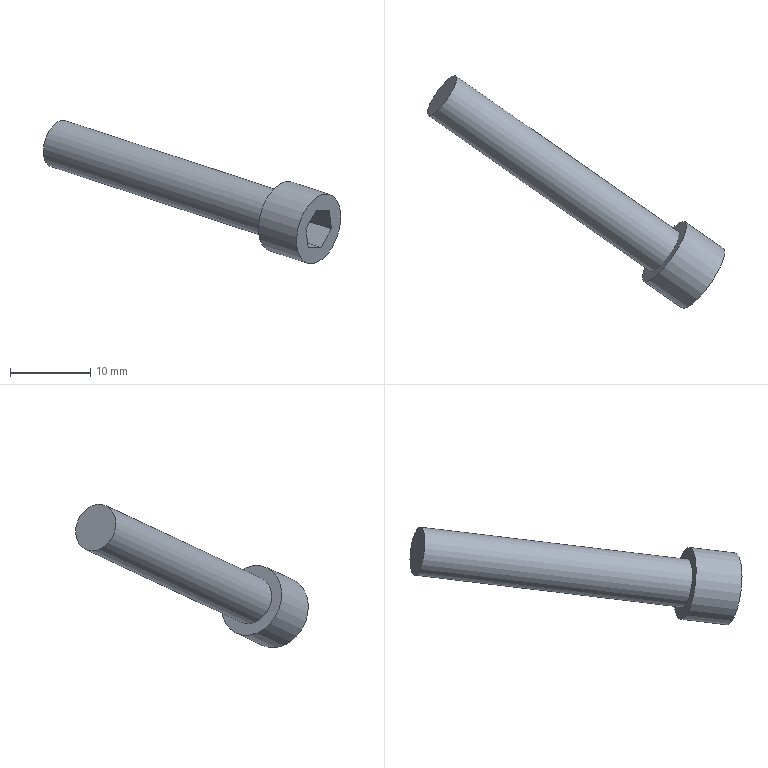Part | NX | features solid 2 | 1 solid | 12 faces | box 37.027 x 28.959 x 17.856 mm | volume 1299 mm3 | plane 10 | cylinder 2 | commonest cylinder face diameters 6 x1 9 x1
STEP:
#1=CARTESIAN_POINT('',(-602.734,262.281,39.067));
#2=VERTEX_POINT('',#1);
#3=CARTESIAN_POINT('',(-603.02,260.79,41.385));
#4=VERTEX_POINT('',#3);
#5=CARTESIAN_POINT('',(-602.877,261.535,40.226));
#6=DIRECTION('',(-0.1032,-0.5381,0.8365));
#7=VECTOR('',#6,1000.);
#8=LINE('',#5,#7);
#9=EDGE_CURVE('',#2,#4,#8,.T.);
#10=ORIENTED_EDGE('',*,*,#9,.T.);
#11=CARTESIAN_POINT('',(-601.716,261.568,43.703));
#12=VERTEX_POINT('',#11);
#13=CARTESIAN_POINT('',(-602.368,261.179,42.544));
#14=DIRECTION('',(0.4704,0.281,0.8365));
#15=VECTOR('',#14,1000.);
#16=LINE('',#13,#15);
#17=EDGE_CURVE('',#4,#12,#16,.T.);
#18=ORIENTED_EDGE('',*,*,#17,.T.);
#19=CARTESIAN_POINT('',(-600.127,263.838,43.703));
#20=VERTEX_POINT('',#19);
#21=CARTESIAN_POINT('',(-600.921,262.703,43.703));
#22=DIRECTION('',(0.5736,0.8192,0.));
#23=VECTOR('',#22,1000.);
#24=LINE('',#21,#23);
#25=EDGE_CURVE('',#12,#20,#24,.T.);
#26=ORIENTED_EDGE('',*,*,#25,.T.);
#27=CARTESIAN_POINT('',(-599.841,265.33,41.385));
#28=VERTEX_POINT('',#27);
#29=CARTESIAN_POINT('',(-599.984,264.584,42.544));
#30=DIRECTION('',(0.1032,0.5381,-0.8365));
#31=VECTOR('',#30,1000.);
#32=LINE('',#29,#31);
#33=EDGE_CURVE('',#20,#28,#32,.T.);
#34=ORIENTED_EDGE('',*,*,#33,.T.);
#35=CARTESIAN_POINT('',(-601.144,264.551,39.067));
#36=VERTEX_POINT('',#35);
#37=CARTESIAN_POINT('',(-600.492,264.94,40.226));
#38=DIRECTION('',(-0.4704,-0.281,-0.8365));
#39=VECTOR('',#38,1000.);
#40=LINE('',#37,#39);
#41=EDGE_CURVE('',#28,#36,#40,.T.);
#42=ORIENTED_EDGE('',*,*,#41,.T.);
#43=CARTESIAN_POINT('',(-601.939,263.416,39.067));
#44=DIRECTION('',(-0.5736,-0.8192,0.));
#45=VECTOR('',#44,1000.);
#46=LINE('',#43,#45);
#47=EDGE_CURVE('',#36,#2,#46,.T.);
#48=ORIENTED_EDGE('',*,*,#47,.T.);
#49=EDGE_LOOP('',(#10,#18,#26,#34,#42,#48));
#50=FACE_BOUND('',#49,.T.);
#51=CARTESIAN_POINT('',(-598.849,266.746,41.385));
#52=VERTEX_POINT('',#51);
#53=CARTESIAN_POINT('',(-601.43,263.06,41.385));
#54=DIRECTION('',(0.7912,-0.554,-0.2588));
#55=DIRECTION('',(0.5736,0.8192,0.));
#56=AXIS2_PLACEMENT_3D('',#53,#54,#55);
#57=CIRCLE('',#56,4.5);
#58=EDGE_CURVE('',#52,#52,#57,.T.);
#59=ORIENTED_EDGE('',*,*,#58,.T.);
#60=EDGE_LOOP('',(#59));
#61=FACE_BOUND('',#60,.T.);
#62=CARTESIAN_POINT('',(-601.43,263.06,41.385));
#63=DIRECTION('',(0.7912,-0.554,-0.2588));
#64=DIRECTION('',(-0.5736,-0.8192,0.));
#65=AXIS2_PLACEMENT_3D('',#62,#63,#64);
#66=PLANE('',#65);
#67=ADVANCED_FACE('',(#50,#61),#66,.T.);
#68=CARTESIAN_POINT('',(-604.457,268.841,42.938));
#69=VERTEX_POINT('',#68);
#70=CARTESIAN_POINT('',(-606.178,266.384,42.938));
#71=DIRECTION('',(0.7912,-0.554,-0.2588));
#72=DIRECTION('',(0.5736,0.8192,0.));
#73=AXIS2_PLACEMENT_3D('',#70,#71,#72);
#74=CIRCLE('',#73,3.);
#75=EDGE_CURVE('',#69,#69,#74,.T.);
#76=ORIENTED_EDGE('',*,*,#75,.T.);
#77=EDGE_LOOP('',(#76));
#78=FACE_BOUND('',#77,.T.);
#79=CARTESIAN_POINT('',(-608.759,262.698,42.938));
#80=VERTEX_POINT('',#79);
#81=CARTESIAN_POINT('',(-606.178,266.384,42.938));
#82=DIRECTION('',(-0.7912,0.554,0.2588));
#83=DIRECTION('',(-0.5736,-0.8192,0.));
#84=AXIS2_PLACEMENT_3D('',#81,#82,#83);
#85=CIRCLE('',#84,4.5);
#86=EDGE_CURVE('',#80,#80,#85,.T.);
#87=ORIENTED_EDGE('',*,*,#86,.T.);
#88=EDGE_LOOP('',(#87));
#89=FACE_BOUND('',#88,.T.);
#90=CARTESIAN_POINT('',(-606.178,266.384,42.938));
#91=DIRECTION('',(-0.7912,0.554,0.2588));
#92=DIRECTION('',(0.5736,0.8192,0.));
#93=AXIS2_PLACEMENT_3D('',#90,#91,#92);
#94=PLANE('',#93);
#95=ADVANCED_FACE('',(#78,#89),#94,.T.);
#96=ORIENTED_EDGE('',*,*,#58,.F.);
#97=EDGE_LOOP('',(#96));
#98=FACE_BOUND('',#97,.T.);
#99=ORIENTED_EDGE('',*,*,#86,.F.);
#100=EDGE_LOOP('',(#99));
#101=FACE_BOUND('',#100,.T.);
#102=CARTESIAN_POINT('',(-606.178,266.384,42.938));
#103=DIRECTION('',(0.7912,-0.554,-0.2588));
#104=DIRECTION('',(-0.5736,-0.8192,0.));
#105=AXIS2_PLACEMENT_3D('',#102,#103,#104);
#106=CYLINDRICAL_SURFACE('',#105,4.5);
#107=ADVANCED_FACE('',(#98,#101),#106,.T.);
#108=ORIENTED_EDGE('',*,*,#9,.F.);
#109=CARTESIAN_POINT('',(-605.582,264.275,39.999));
#110=VERTEX_POINT('',#109);
#111=CARTESIAN_POINT('',(-605.582,264.275,39.999));
#112=DIRECTION('',(0.7912,-0.554,-0.2588));
#113=VECTOR('',#112,1000.);
#114=LINE('',#111,#113);
#115=EDGE_CURVE('',#110,#2,#114,.T.);
#116=ORIENTED_EDGE('',*,*,#115,.F.);
#117=CARTESIAN_POINT('',(-605.868,262.784,42.317));
#118=VERTEX_POINT('',#117);
#119=CARTESIAN_POINT('',(-605.582,264.275,39.999));
#120=DIRECTION('',(-0.1032,-0.5381,0.8365));
#121=VECTOR('',#120,1000.);
#122=LINE('',#119,#121);
#123=EDGE_CURVE('',#110,#118,#122,.T.);
#124=ORIENTED_EDGE('',*,*,#123,.T.);
#125=CARTESIAN_POINT('',(-605.868,262.784,42.317));
#126=DIRECTION('',(0.7912,-0.554,-0.2588));
#127=VECTOR('',#126,1000.);
#128=LINE('',#125,#127);
#129=EDGE_CURVE('',#118,#4,#128,.T.);
#130=ORIENTED_EDGE('',*,*,#129,.T.);
#131=EDGE_LOOP('',(#108,#116,#124,#130));
#132=FACE_BOUND('',#131,.T.);
#133=CARTESIAN_POINT('',(-603.352,261.868,40.381));
#134=DIRECTION('',(-0.6027,-0.6352,-0.483));
#135=DIRECTION('',(-0.7254,0.6883,0.));
#136=AXIS2_PLACEMENT_3D('',#133,#134,#135);
#137=PLANE('',#136);
#138=ADVANCED_FACE('',(#132),#137,.F.);
#139=ORIENTED_EDGE('',*,*,#47,.F.);
#140=CARTESIAN_POINT('',(-603.993,266.546,39.999));
#141=VERTEX_POINT('',#140);
#142=CARTESIAN_POINT('',(-603.993,266.546,39.999));
#143=DIRECTION('',(0.7912,-0.554,-0.2588));
#144=VECTOR('',#143,1000.);
#145=LINE('',#142,#144);
#146=EDGE_CURVE('',#141,#36,#145,.T.);
#147=ORIENTED_EDGE('',*,*,#146,.F.);
#148=CARTESIAN_POINT('',(-603.993,266.546,39.999));
#149=DIRECTION('',(-0.5736,-0.8192,0.));
#150=VECTOR('',#149,1000.);
#151=LINE('',#148,#150);
#152=EDGE_CURVE('',#141,#110,#151,.T.);
#153=ORIENTED_EDGE('',*,*,#152,.T.);
#154=ORIENTED_EDGE('',*,*,#115,.T.);
#155=EDGE_LOOP('',(#139,#147,#153,#154));
#156=FACE_BOUND('',#155,.T.);
#157=CARTESIAN_POINT('',(-602.414,263.748,39.222));
#158=DIRECTION('',(-0.212,0.1485,-0.9659));
#159=DIRECTION('',(-0.1706,0.9676,0.1862));
#160=AXIS2_PLACEMENT_3D('',#157,#158,#159);
#161=PLANE('',#160);
#162=ADVANCED_FACE('',(#156),#161,.F.);
#163=ORIENTED_EDGE('',*,*,#41,.F.);
#164=CARTESIAN_POINT('',(-602.689,267.324,42.317));
#165=VERTEX_POINT('',#164);
#166=CARTESIAN_POINT('',(-602.689,267.324,42.317));
#167=DIRECTION('',(0.7912,-0.554,-0.2588));
#168=VECTOR('',#167,1000.);
#169=LINE('',#166,#168);
#170=EDGE_CURVE('',#165,#28,#169,.T.);
#171=ORIENTED_EDGE('',*,*,#170,.F.);
#172=CARTESIAN_POINT('',(-602.689,267.324,42.317));
#173=DIRECTION('',(-0.4704,-0.281,-0.8365));
#174=VECTOR('',#173,1000.);
#175=LINE('',#172,#174);
#176=EDGE_CURVE('',#165,#141,#175,.T.);
#177=ORIENTED_EDGE('',*,*,#176,.T.);
#178=ORIENTED_EDGE('',*,*,#146,.T.);
#179=EDGE_LOOP('',(#163,#171,#177,#178));
#180=FACE_BOUND('',#179,.T.);
#181=CARTESIAN_POINT('',(-600.967,265.273,40.381));
#182=DIRECTION('',(0.3907,0.7836,-0.483));
#183=DIRECTION('',(0.8949,-0.4462,0.));
#184=AXIS2_PLACEMENT_3D('',#181,#182,#183);
#185=PLANE('',#184);
#186=ADVANCED_FACE('',(#180),#185,.F.);
#187=ORIENTED_EDGE('',*,*,#33,.F.);
#188=CARTESIAN_POINT('',(-602.975,265.833,44.635));
#189=VERTEX_POINT('',#188);
#190=CARTESIAN_POINT('',(-602.975,265.833,44.635));
#191=DIRECTION('',(0.7912,-0.554,-0.2588));
#192=VECTOR('',#191,1000.);
#193=LINE('',#190,#192);
#194=EDGE_CURVE('',#189,#20,#193,.T.);
#195=ORIENTED_EDGE('',*,*,#194,.F.);
#196=CARTESIAN_POINT('',(-602.975,265.833,44.635));
#197=DIRECTION('',(0.1032,0.5381,-0.8365));
#198=VECTOR('',#197,1000.);
#199=LINE('',#196,#198);
#200=EDGE_CURVE('',#189,#165,#199,.T.);
#201=ORIENTED_EDGE('',*,*,#200,.T.);
#202=ORIENTED_EDGE('',*,*,#170,.T.);
#203=EDGE_LOOP('',(#187,#195,#201,#202));
#204=FACE_BOUND('',#203,.T.);
#205=CARTESIAN_POINT('',(-600.458,264.917,42.7));
#206=DIRECTION('',(0.6027,0.6352,0.483));
#207=DIRECTION('',(0.7254,-0.6883,0.));
#208=AXIS2_PLACEMENT_3D('',#205,#206,#207);
#209=PLANE('',#208);
#210=ADVANCED_FACE('',(#204),#209,.F.);
#211=ORIENTED_EDGE('',*,*,#25,.F.);
#212=CARTESIAN_POINT('',(-604.565,263.563,44.635));
#213=VERTEX_POINT('',#212);
#214=CARTESIAN_POINT('',(-604.565,263.563,44.635));
#215=DIRECTION('',(0.7912,-0.554,-0.2588));
#216=VECTOR('',#215,1000.);
#217=LINE('',#214,#216);
#218=EDGE_CURVE('',#213,#12,#217,.T.);
#219=ORIENTED_EDGE('',*,*,#218,.F.);
#220=CARTESIAN_POINT('',(-604.565,263.563,44.635));
#221=DIRECTION('',(0.5736,0.8192,0.));
#222=VECTOR('',#221,1000.);
#223=LINE('',#220,#222);
#224=EDGE_CURVE('',#213,#189,#223,.T.);
#225=ORIENTED_EDGE('',*,*,#224,.T.);
#226=ORIENTED_EDGE('',*,*,#194,.T.);
#227=EDGE_LOOP('',(#211,#219,#225,#226));
#228=FACE_BOUND('',#227,.T.);
#229=CARTESIAN_POINT('',(-601.396,263.036,43.859));
#230=DIRECTION('',(0.212,-0.1485,0.9659));
#231=DIRECTION('',(-0.9676,-0.1706,0.1862));
#232=AXIS2_PLACEMENT_3D('',#229,#230,#231);
#233=PLANE('',#232);
#234=ADVANCED_FACE('',(#228),#233,.F.);
#235=ORIENTED_EDGE('',*,*,#17,.F.);
#236=ORIENTED_EDGE('',*,*,#129,.F.);
#237=CARTESIAN_POINT('',(-605.868,262.784,42.317));
#238=DIRECTION('',(0.4704,0.281,0.8365));
#239=VECTOR('',#238,1000.);
#240=LINE('',#237,#239);
#241=EDGE_CURVE('',#118,#213,#240,.T.);
#242=ORIENTED_EDGE('',*,*,#241,.T.);
#243=ORIENTED_EDGE('',*,*,#218,.T.);
#244=EDGE_LOOP('',(#235,#236,#242,#243));
#245=FACE_BOUND('',#244,.T.);
#246=CARTESIAN_POINT('',(-602.843,261.511,42.7));
#247=DIRECTION('',(-0.3907,-0.7836,0.483));
#248=DIRECTION('',(-0.8949,0.4462,0.));
#249=AXIS2_PLACEMENT_3D('',#246,#247,#248);
#250=PLANE('',#249);
#251=ADVANCED_FACE('',(#245),#250,.F.);
#252=ORIENTED_EDGE('',*,*,#241,.F.);
#253=ORIENTED_EDGE('',*,*,#123,.F.);
#254=ORIENTED_EDGE('',*,*,#152,.F.);
#255=ORIENTED_EDGE('',*,*,#176,.F.);
#256=ORIENTED_EDGE('',*,*,#200,.F.);
#257=ORIENTED_EDGE('',*,*,#224,.F.);
#258=EDGE_LOOP('',(#252,#253,#254,#255,#256,#257));
#259=FACE_BOUND('',#258,.T.);
#260=CARTESIAN_POINT('',(-604.279,265.054,42.317));
#261=DIRECTION('',(-0.7912,0.554,0.2588));
#262=DIRECTION('',(0.5736,0.8192,0.));
#263=AXIS2_PLACEMENT_3D('',#260,#261,#262);
#264=PLANE('',#263);
#265=ADVANCED_FACE('',(#259),#264,.F.);
#266=CARTESIAN_POINT('',(-632.15,288.232,51.997));
#267=VERTEX_POINT('',#266);
#268=CARTESIAN_POINT('',(-633.871,285.775,51.997));
#269=DIRECTION('',(0.7912,-0.554,-0.2588));
#270=DIRECTION('',(0.5736,0.8192,0.));
#271=AXIS2_PLACEMENT_3D('',#268,#269,#270);
#272=CIRCLE('',#271,3.);
#273=EDGE_CURVE('',#267,#267,#272,.F.);
#274=ORIENTED_EDGE('',*,*,#273,.T.);
#275=EDGE_LOOP('',(#274));
#276=FACE_BOUND('',#275,.T.);
#277=CARTESIAN_POINT('',(-633.871,285.775,51.997));
#278=DIRECTION('',(-0.7912,0.554,0.2588));
#279=DIRECTION('',(0.5736,0.8192,0.));
#280=AXIS2_PLACEMENT_3D('',#277,#278,#279);
#281=PLANE('',#280);
#282=ADVANCED_FACE('',(#276),#281,.T.);
#283=ORIENTED_EDGE('',*,*,#273,.F.);
#284=EDGE_LOOP('',(#283));
#285=FACE_BOUND('',#284,.T.);
#286=ORIENTED_EDGE('',*,*,#75,.F.);
#287=EDGE_LOOP('',(#286));
#288=FACE_BOUND('',#287,.T.);
#289=CARTESIAN_POINT('',(-606.178,266.384,42.938));
#290=DIRECTION('',(-0.7912,0.554,0.2588));
#291=DIRECTION('',(0.5736,0.8192,0.));
#292=AXIS2_PLACEMENT_3D('',#289,#290,#291);
#293=CYLINDRICAL_SURFACE('',#292,3.);
#294=ADVANCED_FACE('',(#285,#288),#293,.T.);
#295=CLOSED_SHELL('',(#67,#95,#107,#138,#162,#186,#210,#234,#251,#265,#282,#294));
#296=MANIFOLD_SOLID_BREP('',#295);
#297=(LENGTH_UNIT()NAMED_UNIT(*)SI_UNIT(.MILLI.,.METRE.));
#298=UNCERTAINTY_MEASURE_WITH_UNIT(LENGTH_MEASURE(0.00001),#297,'','');
#299=(NAMED_UNIT(*)PLANE_ANGLE_UNIT()SI_UNIT($,.RADIAN.));
#300=(NAMED_UNIT(*)SI_UNIT($,.STERADIAN.)SOLID_ANGLE_UNIT());
#301=(GEOMETRIC_REPRESENTATION_CONTEXT(3)GLOBAL_UNCERTAINTY_ASSIGNED_CONTEXT((#298))GLOBAL_UNIT_ASSIGNED_CONTEXT((#297,#299,#300))REPRESENTATION_CONTEXT('',''));
#302=ADVANCED_BREP_SHAPE_REPRESENTATION('',(#296),#301);